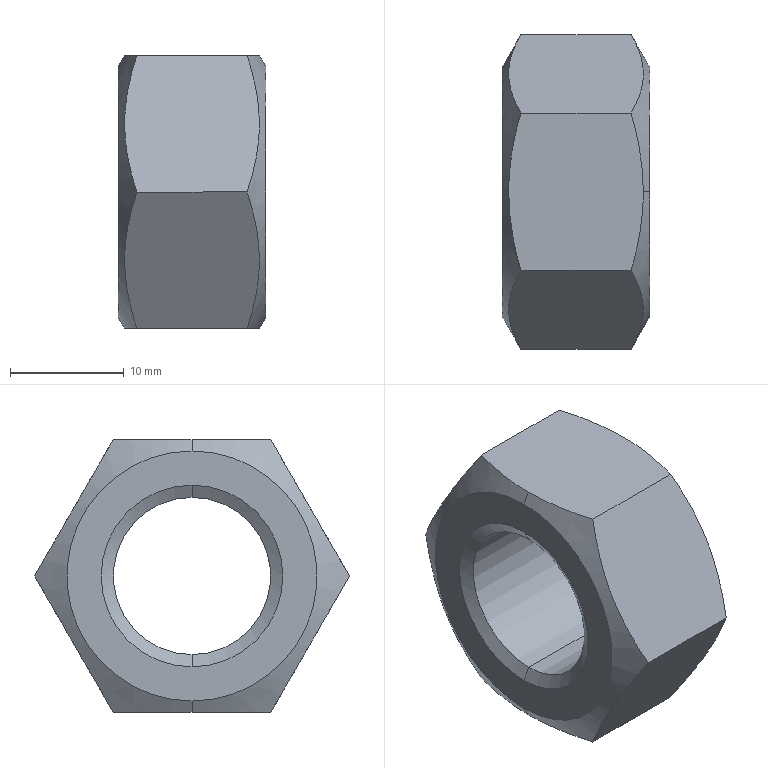Part | STEP file | DIN 555 - replaced by DIN EN 24034 M16 | 1 solid | 18 faces | box 13 x 27.713 x 24 mm | volume 4374 mm3 | cone 8 | plane 8 | cylinder 2 | commonest cylinder face diameters 13.835 x2